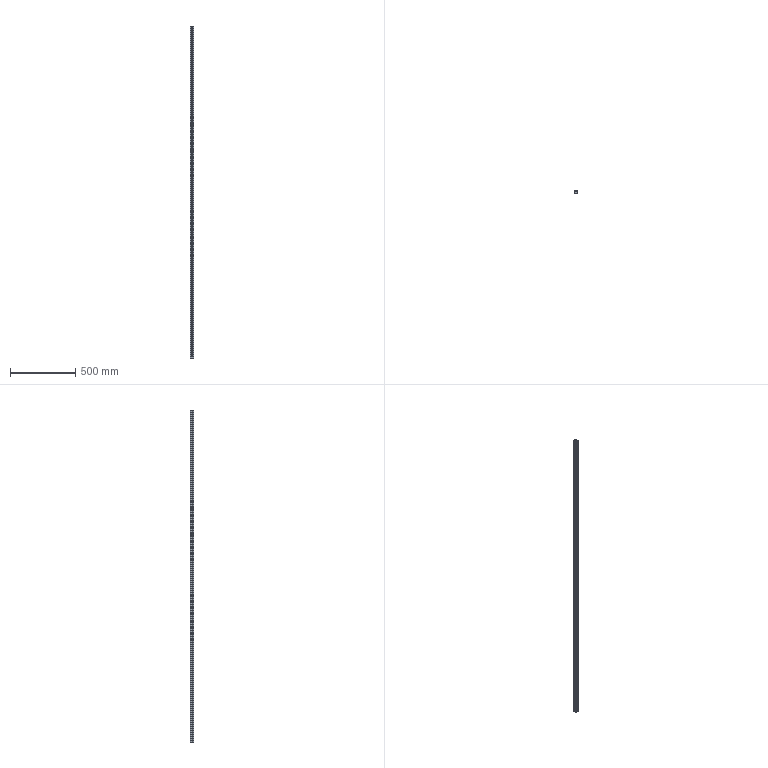Part | STEP file | _IBC23-45-1500_001 | 1 solid | 178 faces | box 28 x 26 x 2540 mm | volume 1504984 mm3 | plane 102 | cylinder 76 | commonest cylinder face diameters 9 x36 14 x36 6.2 x4